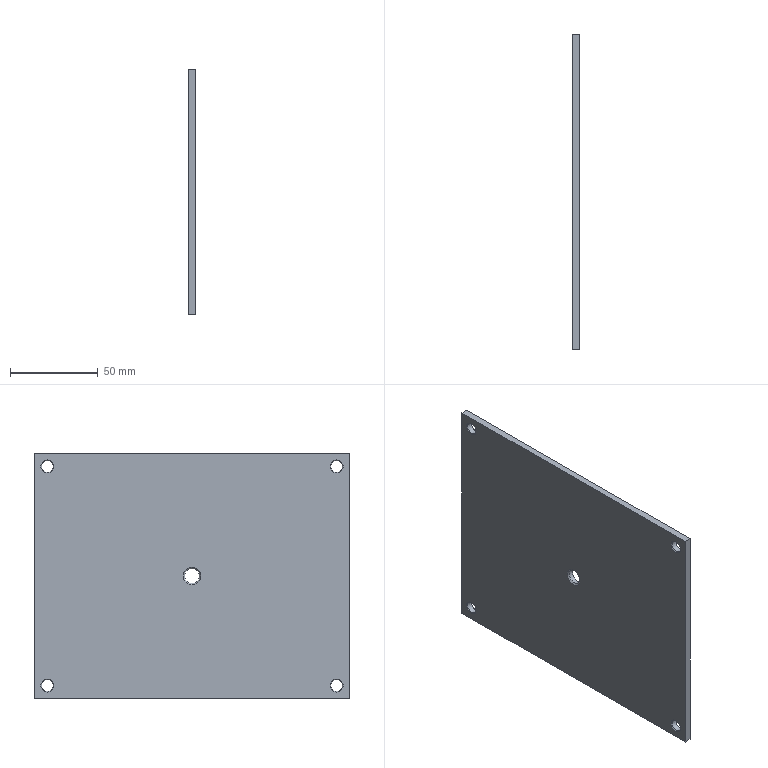Part | NX | 1 solid | 21 faces | box 4 x 180 x 140 mm | volume 99996 mm3 | cone 10 | plane 6 | cylinder 5 | commonest cylinder face diameters 6.6 x4 8.5 x1
STEP:
#1=CARTESIAN_POINT('',(2.,90.,-70.));
#2=VERTEX_POINT('',#1);
#3=CARTESIAN_POINT('',(2.,-90.,-70.));
#4=VERTEX_POINT('',#3);
#5=CARTESIAN_POINT('',(2.,90.,-70.));
#6=DIRECTION('',(0.,-1.,0.));
#7=VECTOR('',#6,1.);
#8=LINE('',#5,#7);
#9=EDGE_CURVE('',#2,#4,#8,.T.);
#10=ORIENTED_EDGE('',*,*,#9,.F.);
#11=CARTESIAN_POINT('',(6.,90.,-70.));
#12=VERTEX_POINT('',#11);
#13=CARTESIAN_POINT('',(6.,90.,-70.));
#14=DIRECTION('',(-1.,0.,0.));
#15=VECTOR('',#14,1.);
#16=LINE('',#13,#15);
#17=EDGE_CURVE('',#12,#2,#16,.T.);
#18=ORIENTED_EDGE('',*,*,#17,.F.);
#19=CARTESIAN_POINT('',(6.,-90.,-70.));
#20=VERTEX_POINT('',#19);
#21=CARTESIAN_POINT('',(6.,90.,-70.));
#22=DIRECTION('',(0.,-1.,0.));
#23=VECTOR('',#22,1.);
#24=LINE('',#21,#23);
#25=EDGE_CURVE('',#12,#20,#24,.T.);
#26=ORIENTED_EDGE('',*,*,#25,.T.);
#27=CARTESIAN_POINT('',(6.,-90.,-70.));
#28=DIRECTION('',(-1.,0.,0.));
#29=VECTOR('',#28,1.);
#30=LINE('',#27,#29);
#31=EDGE_CURVE('',#20,#4,#30,.T.);
#32=ORIENTED_EDGE('',*,*,#31,.T.);
#33=EDGE_LOOP('',(#10,#18,#26,#32));
#34=FACE_OUTER_BOUND('',#33,.T.);
#35=CARTESIAN_POINT('',(6.,90.,-70.));
#36=DIRECTION('',(0.,0.,-1.));
#37=DIRECTION('',(0.,-1.,0.));
#38=AXIS2_PLACEMENT_3D('',#35,#36,#37);
#39=PLANE('',#38);
#40=ADVANCED_FACE('',(#34),#39,.T.);
#41=CARTESIAN_POINT('',(2.,-90.,70.));
#42=VERTEX_POINT('',#41);
#43=CARTESIAN_POINT('',(2.,-90.,-70.));
#44=DIRECTION('',(0.,0.,1.));
#45=VECTOR('',#44,1.);
#46=LINE('',#43,#45);
#47=EDGE_CURVE('',#4,#42,#46,.T.);
#48=ORIENTED_EDGE('',*,*,#47,.F.);
#49=ORIENTED_EDGE('',*,*,#31,.F.);
#50=CARTESIAN_POINT('',(6.,-90.,70.));
#51=VERTEX_POINT('',#50);
#52=CARTESIAN_POINT('',(6.,-90.,-70.));
#53=DIRECTION('',(0.,0.,1.));
#54=VECTOR('',#53,1.);
#55=LINE('',#52,#54);
#56=EDGE_CURVE('',#20,#51,#55,.T.);
#57=ORIENTED_EDGE('',*,*,#56,.T.);
#58=CARTESIAN_POINT('',(6.,-90.,70.));
#59=DIRECTION('',(-1.,0.,0.));
#60=VECTOR('',#59,1.);
#61=LINE('',#58,#60);
#62=EDGE_CURVE('',#51,#42,#61,.T.);
#63=ORIENTED_EDGE('',*,*,#62,.T.);
#64=EDGE_LOOP('',(#48,#49,#57,#63));
#65=FACE_OUTER_BOUND('',#64,.T.);
#66=CARTESIAN_POINT('',(6.,-90.,-70.));
#67=DIRECTION('',(0.,-1.,0.));
#68=DIRECTION('',(0.,0.,1.));
#69=AXIS2_PLACEMENT_3D('',#66,#67,#68);
#70=PLANE('',#69);
#71=ADVANCED_FACE('',(#65),#70,.T.);
#72=CARTESIAN_POINT('',(2.,90.,70.));
#73=VERTEX_POINT('',#72);
#74=CARTESIAN_POINT('',(2.,-90.,70.));
#75=DIRECTION('',(0.,1.,0.));
#76=VECTOR('',#75,1.);
#77=LINE('',#74,#76);
#78=EDGE_CURVE('',#42,#73,#77,.T.);
#79=ORIENTED_EDGE('',*,*,#78,.F.);
#80=ORIENTED_EDGE('',*,*,#62,.F.);
#81=CARTESIAN_POINT('',(6.,90.,70.));
#82=VERTEX_POINT('',#81);
#83=CARTESIAN_POINT('',(6.,-90.,70.));
#84=DIRECTION('',(0.,1.,0.));
#85=VECTOR('',#84,1.);
#86=LINE('',#83,#85);
#87=EDGE_CURVE('',#51,#82,#86,.T.);
#88=ORIENTED_EDGE('',*,*,#87,.T.);
#89=CARTESIAN_POINT('',(6.,90.,70.));
#90=DIRECTION('',(-1.,0.,0.));
#91=VECTOR('',#90,1.);
#92=LINE('',#89,#91);
#93=EDGE_CURVE('',#82,#73,#92,.T.);
#94=ORIENTED_EDGE('',*,*,#93,.T.);
#95=EDGE_LOOP('',(#79,#80,#88,#94));
#96=FACE_OUTER_BOUND('',#95,.T.);
#97=CARTESIAN_POINT('',(6.,-90.,70.));
#98=DIRECTION('',(0.,0.,1.));
#99=DIRECTION('',(0.,1.,0.));
#100=AXIS2_PLACEMENT_3D('',#97,#98,#99);
#101=PLANE('',#100);
#102=ADVANCED_FACE('',(#96),#101,.T.);
#103=CARTESIAN_POINT('',(2.,90.,70.));
#104=DIRECTION('',(0.,0.,-1.));
#105=VECTOR('',#104,1.);
#106=LINE('',#103,#105);
#107=EDGE_CURVE('',#73,#2,#106,.T.);
#108=ORIENTED_EDGE('',*,*,#107,.F.);
#109=ORIENTED_EDGE('',*,*,#93,.F.);
#110=CARTESIAN_POINT('',(6.,90.,70.));
#111=DIRECTION('',(0.,0.,-1.));
#112=VECTOR('',#111,1.);
#113=LINE('',#110,#112);
#114=EDGE_CURVE('',#82,#12,#113,.T.);
#115=ORIENTED_EDGE('',*,*,#114,.T.);
#116=ORIENTED_EDGE('',*,*,#17,.T.);
#117=EDGE_LOOP('',(#108,#109,#115,#116));
#118=FACE_OUTER_BOUND('',#117,.T.);
#119=CARTESIAN_POINT('',(6.,90.,70.));
#120=DIRECTION('',(0.,1.,0.));
#121=DIRECTION('',(0.,0.,-1.));
#122=AXIS2_PLACEMENT_3D('',#119,#120,#121);
#123=PLANE('',#122);
#124=ADVANCED_FACE('',(#118),#123,.T.);
#125=CARTESIAN_POINT('',(6.,0.,5.));
#126=VERTEX_POINT('',#125);
#127=CARTESIAN_POINT('',(6.,0.,0.));
#128=DIRECTION('',(-1.,0.,0.));
#129=DIRECTION('',(0.,0.,1.));
#130=AXIS2_PLACEMENT_3D('',#127,#128,#129);
#131=CIRCLE('',#130,5.);
#132=EDGE_CURVE('',#126,#126,#131,.T.);
#133=ORIENTED_EDGE('',*,*,#132,.T.);
#134=EDGE_LOOP('',(#133));
#135=FACE_BOUND('',#134,.T.);
#136=CARTESIAN_POINT('',(6.,82.5,66.2));
#137=VERTEX_POINT('',#136);
#138=CARTESIAN_POINT('',(6.,82.5,62.5));
#139=DIRECTION('',(-1.,0.,0.));
#140=DIRECTION('',(0.,0.,1.));
#141=AXIS2_PLACEMENT_3D('',#138,#139,#140);
#142=CIRCLE('',#141,3.7);
#143=EDGE_CURVE('',#137,#137,#142,.T.);
#144=ORIENTED_EDGE('',*,*,#143,.T.);
#145=EDGE_LOOP('',(#144));
#146=FACE_BOUND('',#145,.T.);
#147=CARTESIAN_POINT('',(6.,82.5,-58.8));
#148=VERTEX_POINT('',#147);
#149=CARTESIAN_POINT('',(6.,82.5,-62.5));
#150=DIRECTION('',(-1.,0.,0.));
#151=DIRECTION('',(0.,0.,1.));
#152=AXIS2_PLACEMENT_3D('',#149,#150,#151);
#153=CIRCLE('',#152,3.7);
#154=EDGE_CURVE('',#148,#148,#153,.T.);
#155=ORIENTED_EDGE('',*,*,#154,.T.);
#156=EDGE_LOOP('',(#155));
#157=FACE_BOUND('',#156,.T.);
#158=CARTESIAN_POINT('',(6.,-82.5,66.2));
#159=VERTEX_POINT('',#158);
#160=CARTESIAN_POINT('',(6.,-82.5,62.5));
#161=DIRECTION('',(-1.,0.,0.));
#162=DIRECTION('',(0.,0.,1.));
#163=AXIS2_PLACEMENT_3D('',#160,#161,#162);
#164=CIRCLE('',#163,3.7);
#165=EDGE_CURVE('',#159,#159,#164,.T.);
#166=ORIENTED_EDGE('',*,*,#165,.T.);
#167=EDGE_LOOP('',(#166));
#168=FACE_BOUND('',#167,.T.);
#169=CARTESIAN_POINT('',(6.,-82.5,-58.8));
#170=VERTEX_POINT('',#169);
#171=CARTESIAN_POINT('',(6.,-82.5,-62.5));
#172=DIRECTION('',(-1.,0.,0.));
#173=DIRECTION('',(0.,0.,1.));
#174=AXIS2_PLACEMENT_3D('',#171,#172,#173);
#175=CIRCLE('',#174,3.7);
#176=EDGE_CURVE('',#170,#170,#175,.T.);
#177=ORIENTED_EDGE('',*,*,#176,.T.);
#178=EDGE_LOOP('',(#177));
#179=FACE_BOUND('',#178,.T.);
#180=ORIENTED_EDGE('',*,*,#25,.F.);
#181=ORIENTED_EDGE('',*,*,#114,.F.);
#182=ORIENTED_EDGE('',*,*,#87,.F.);
#183=ORIENTED_EDGE('',*,*,#56,.F.);
#184=EDGE_LOOP('',(#180,#181,#182,#183));
#185=FACE_BOUND('',#184,.T.);
#186=CARTESIAN_POINT('',(6.,0.,0.));
#187=DIRECTION('',(-1.,0.,0.));
#188=DIRECTION('',(0.,0.,-1.));
#189=AXIS2_PLACEMENT_3D('',#186,#187,#188);
#190=PLANE('',#189);
#191=ADVANCED_FACE('',(#135,#146,#157,#168,#179,#185),#190,.F.);
#192=CARTESIAN_POINT('',(2.,0.,5.));
#193=VERTEX_POINT('',#192);
#194=CARTESIAN_POINT('',(2.,0.,0.));
#195=DIRECTION('',(1.,0.,0.));
#196=DIRECTION('',(0.,0.,1.));
#197=AXIS2_PLACEMENT_3D('',#194,#195,#196);
#198=CIRCLE('',#197,5.);
#199=EDGE_CURVE('',#193,#193,#198,.T.);
#200=ORIENTED_EDGE('',*,*,#199,.T.);
#201=EDGE_LOOP('',(#200));
#202=FACE_BOUND('',#201,.T.);
#203=CARTESIAN_POINT('',(2.,82.5,66.2));
#204=VERTEX_POINT('',#203);
#205=CARTESIAN_POINT('',(2.,82.5,62.5));
#206=DIRECTION('',(1.,0.,0.));
#207=DIRECTION('',(0.,0.,1.));
#208=AXIS2_PLACEMENT_3D('',#205,#206,#207);
#209=CIRCLE('',#208,3.7);
#210=EDGE_CURVE('',#204,#204,#209,.T.);
#211=ORIENTED_EDGE('',*,*,#210,.T.);
#212=EDGE_LOOP('',(#211));
#213=FACE_BOUND('',#212,.T.);
#214=CARTESIAN_POINT('',(2.,82.5,-58.8));
#215=VERTEX_POINT('',#214);
#216=CARTESIAN_POINT('',(2.,82.5,-62.5));
#217=DIRECTION('',(1.,0.,0.));
#218=DIRECTION('',(0.,0.,1.));
#219=AXIS2_PLACEMENT_3D('',#216,#217,#218);
#220=CIRCLE('',#219,3.7);
#221=EDGE_CURVE('',#215,#215,#220,.T.);
#222=ORIENTED_EDGE('',*,*,#221,.T.);
#223=EDGE_LOOP('',(#222));
#224=FACE_BOUND('',#223,.T.);
#225=CARTESIAN_POINT('',(2.,-82.5,66.2));
#226=VERTEX_POINT('',#225);
#227=CARTESIAN_POINT('',(2.,-82.5,62.5));
#228=DIRECTION('',(1.,0.,0.));
#229=DIRECTION('',(0.,0.,1.));
#230=AXIS2_PLACEMENT_3D('',#227,#228,#229);
#231=CIRCLE('',#230,3.7);
#232=EDGE_CURVE('',#226,#226,#231,.T.);
#233=ORIENTED_EDGE('',*,*,#232,.T.);
#234=EDGE_LOOP('',(#233));
#235=FACE_BOUND('',#234,.T.);
#236=CARTESIAN_POINT('',(2.,-82.5,-58.8));
#237=VERTEX_POINT('',#236);
#238=CARTESIAN_POINT('',(2.,-82.5,-62.5));
#239=DIRECTION('',(1.,0.,0.));
#240=DIRECTION('',(0.,0.,1.));
#241=AXIS2_PLACEMENT_3D('',#238,#239,#240);
#242=CIRCLE('',#241,3.7);
#243=EDGE_CURVE('',#237,#237,#242,.T.);
#244=ORIENTED_EDGE('',*,*,#243,.T.);
#245=EDGE_LOOP('',(#244));
#246=FACE_BOUND('',#245,.T.);
#247=ORIENTED_EDGE('',*,*,#9,.T.);
#248=ORIENTED_EDGE('',*,*,#47,.T.);
#249=ORIENTED_EDGE('',*,*,#78,.T.);
#250=ORIENTED_EDGE('',*,*,#107,.T.);
#251=EDGE_LOOP('',(#247,#248,#249,#250));
#252=FACE_BOUND('',#251,.T.);
#253=CARTESIAN_POINT('',(2.,0.,0.));
#254=DIRECTION('',(-1.,0.,0.));
#255=DIRECTION('',(0.,0.,-1.));
#256=AXIS2_PLACEMENT_3D('',#253,#254,#255);
#257=PLANE('',#256);
#258=ADVANCED_FACE('',(#202,#213,#224,#235,#246,#252),#257,.T.);
#259=CARTESIAN_POINT('',(5.6,-82.5,-59.2));
#260=VERTEX_POINT('',#259);
#261=CARTESIAN_POINT('',(5.6,-82.5,-62.5));
#262=DIRECTION('',(1.,0.,0.));
#263=DIRECTION('',(0.,0.,1.));
#264=AXIS2_PLACEMENT_3D('',#261,#262,#263);
#265=CIRCLE('',#264,3.3);
#266=EDGE_CURVE('',#260,#260,#265,.T.);
#267=ORIENTED_EDGE('',*,*,#266,.T.);
#268=EDGE_LOOP('',(#267));
#269=FACE_BOUND('',#268,.T.);
#270=CARTESIAN_POINT('',(2.4,-82.5,-59.2));
#271=VERTEX_POINT('',#270);
#272=CARTESIAN_POINT('',(2.4,-82.5,-62.5));
#273=DIRECTION('',(-1.,0.,0.));
#274=DIRECTION('',(0.,0.,1.));
#275=AXIS2_PLACEMENT_3D('',#272,#273,#274);
#276=CIRCLE('',#275,3.3);
#277=EDGE_CURVE('',#271,#271,#276,.T.);
#278=ORIENTED_EDGE('',*,*,#277,.T.);
#279=EDGE_LOOP('',(#278));
#280=FACE_BOUND('',#279,.T.);
#281=CARTESIAN_POINT('',(0.,-82.5,-62.5));
#282=DIRECTION('',(1.,0.,0.));
#283=DIRECTION('',(0.,0.,1.));
#284=AXIS2_PLACEMENT_3D('',#281,#282,#283);
#285=CYLINDRICAL_SURFACE('',#284,3.3);
#286=ADVANCED_FACE('',(#269,#280),#285,.F.);
#287=ORIENTED_EDGE('',*,*,#243,.F.);
#288=EDGE_LOOP('',(#287));
#289=FACE_BOUND('',#288,.T.);
#290=ORIENTED_EDGE('',*,*,#277,.F.);
#291=EDGE_LOOP('',(#290));
#292=FACE_BOUND('',#291,.T.);
#293=CARTESIAN_POINT('',(2.4,-82.5,-62.5));
#294=DIRECTION('',(-1.,0.,0.));
#295=DIRECTION('',(0.,0.,-1.));
#296=AXIS2_PLACEMENT_3D('',#293,#294,#295);
#297=CONICAL_SURFACE('',#296,3.3,45.);
#298=ADVANCED_FACE('',(#289,#292),#297,.F.);
#299=ORIENTED_EDGE('',*,*,#266,.F.);
#300=EDGE_LOOP('',(#299));
#301=FACE_BOUND('',#300,.T.);
#302=ORIENTED_EDGE('',*,*,#176,.F.);
#303=EDGE_LOOP('',(#302));
#304=FACE_BOUND('',#303,.T.);
#305=CARTESIAN_POINT('',(6.,-82.5,-62.5));
#306=DIRECTION('',(1.,0.,0.));
#307=DIRECTION('',(0.,0.,1.));
#308=AXIS2_PLACEMENT_3D('',#305,#306,#307);
#309=CONICAL_SURFACE('',#308,3.7,45.);
#310=ADVANCED_FACE('',(#301,#304),#309,.F.);
#311=CARTESIAN_POINT('',(5.6,-82.5,65.8));
#312=VERTEX_POINT('',#311);
#313=CARTESIAN_POINT('',(5.6,-82.5,62.5));
#314=DIRECTION('',(1.,0.,0.));
#315=DIRECTION('',(0.,0.,1.));
#316=AXIS2_PLACEMENT_3D('',#313,#314,#315);
#317=CIRCLE('',#316,3.3);
#318=EDGE_CURVE('',#312,#312,#317,.T.);
#319=ORIENTED_EDGE('',*,*,#318,.T.);
#320=EDGE_LOOP('',(#319));
#321=FACE_BOUND('',#320,.T.);
#322=CARTESIAN_POINT('',(2.4,-82.5,65.8));
#323=VERTEX_POINT('',#322);
#324=CARTESIAN_POINT('',(2.4,-82.5,62.5));
#325=DIRECTION('',(-1.,0.,0.));
#326=DIRECTION('',(0.,0.,1.));
#327=AXIS2_PLACEMENT_3D('',#324,#325,#326);
#328=CIRCLE('',#327,3.3);
#329=EDGE_CURVE('',#323,#323,#328,.T.);
#330=ORIENTED_EDGE('',*,*,#329,.T.);
#331=EDGE_LOOP('',(#330));
#332=FACE_BOUND('',#331,.T.);
#333=CARTESIAN_POINT('',(0.,-82.5,62.5));
#334=DIRECTION('',(1.,0.,0.));
#335=DIRECTION('',(0.,0.,1.));
#336=AXIS2_PLACEMENT_3D('',#333,#334,#335);
#337=CYLINDRICAL_SURFACE('',#336,3.3);
#338=ADVANCED_FACE('',(#321,#332),#337,.F.);
#339=ORIENTED_EDGE('',*,*,#232,.F.);
#340=EDGE_LOOP('',(#339));
#341=FACE_BOUND('',#340,.T.);
#342=ORIENTED_EDGE('',*,*,#329,.F.);
#343=EDGE_LOOP('',(#342));
#344=FACE_BOUND('',#343,.T.);
#345=CARTESIAN_POINT('',(2.4,-82.5,62.5));
#346=DIRECTION('',(-1.,0.,0.));
#347=DIRECTION('',(0.,0.,-1.));
#348=AXIS2_PLACEMENT_3D('',#345,#346,#347);
#349=CONICAL_SURFACE('',#348,3.3,45.);
#350=ADVANCED_FACE('',(#341,#344),#349,.F.);
#351=ORIENTED_EDGE('',*,*,#318,.F.);
#352=EDGE_LOOP('',(#351));
#353=FACE_BOUND('',#352,.T.);
#354=ORIENTED_EDGE('',*,*,#165,.F.);
#355=EDGE_LOOP('',(#354));
#356=FACE_BOUND('',#355,.T.);
#357=CARTESIAN_POINT('',(6.,-82.5,62.5));
#358=DIRECTION('',(1.,0.,0.));
#359=DIRECTION('',(0.,0.,1.));
#360=AXIS2_PLACEMENT_3D('',#357,#358,#359);
#361=CONICAL_SURFACE('',#360,3.7,45.);
#362=ADVANCED_FACE('',(#353,#356),#361,.F.);
#363=CARTESIAN_POINT('',(5.6,82.5,-59.2));
#364=VERTEX_POINT('',#363);
#365=CARTESIAN_POINT('',(5.6,82.5,-62.5));
#366=DIRECTION('',(1.,0.,0.));
#367=DIRECTION('',(0.,0.,1.));
#368=AXIS2_PLACEMENT_3D('',#365,#366,#367);
#369=CIRCLE('',#368,3.3);
#370=EDGE_CURVE('',#364,#364,#369,.T.);
#371=ORIENTED_EDGE('',*,*,#370,.T.);
#372=EDGE_LOOP('',(#371));
#373=FACE_BOUND('',#372,.T.);
#374=CARTESIAN_POINT('',(2.4,82.5,-59.2));
#375=VERTEX_POINT('',#374);
#376=CARTESIAN_POINT('',(2.4,82.5,-62.5));
#377=DIRECTION('',(-1.,0.,0.));
#378=DIRECTION('',(0.,0.,1.));
#379=AXIS2_PLACEMENT_3D('',#376,#377,#378);
#380=CIRCLE('',#379,3.3);
#381=EDGE_CURVE('',#375,#375,#380,.T.);
#382=ORIENTED_EDGE('',*,*,#381,.T.);
#383=EDGE_LOOP('',(#382));
#384=FACE_BOUND('',#383,.T.);
#385=CARTESIAN_POINT('',(0.,82.5,-62.5));
#386=DIRECTION('',(1.,0.,0.));
#387=DIRECTION('',(0.,0.,1.));
#388=AXIS2_PLACEMENT_3D('',#385,#386,#387);
#389=CYLINDRICAL_SURFACE('',#388,3.3);
#390=ADVANCED_FACE('',(#373,#384),#389,.F.);
#391=ORIENTED_EDGE('',*,*,#221,.F.);
#392=EDGE_LOOP('',(#391));
#393=FACE_BOUND('',#392,.T.);
#394=ORIENTED_EDGE('',*,*,#381,.F.);
#395=EDGE_LOOP('',(#394));
#396=FACE_BOUND('',#395,.T.);
#397=CARTESIAN_POINT('',(2.4,82.5,-62.5));
#398=DIRECTION('',(-1.,0.,0.));
#399=DIRECTION('',(0.,0.,-1.));
#400=AXIS2_PLACEMENT_3D('',#397,#398,#399);
#401=CONICAL_SURFACE('',#400,3.3,45.);
#402=ADVANCED_FACE('',(#393,#396),#401,.F.);
#403=ORIENTED_EDGE('',*,*,#370,.F.);
#404=EDGE_LOOP('',(#403));
#405=FACE_BOUND('',#404,.T.);
#406=ORIENTED_EDGE('',*,*,#154,.F.);
#407=EDGE_LOOP('',(#406));
#408=FACE_BOUND('',#407,.T.);
#409=CARTESIAN_POINT('',(6.,82.5,-62.5));
#410=DIRECTION('',(1.,0.,0.));
#411=DIRECTION('',(0.,0.,1.));
#412=AXIS2_PLACEMENT_3D('',#409,#410,#411);
#413=CONICAL_SURFACE('',#412,3.7,45.);
#414=ADVANCED_FACE('',(#405,#408),#413,.F.);
#415=CARTESIAN_POINT('',(5.6,82.5,65.8));
#416=VERTEX_POINT('',#415);
#417=CARTESIAN_POINT('',(5.6,82.5,62.5));
#418=DIRECTION('',(1.,0.,0.));
#419=DIRECTION('',(0.,0.,1.));
#420=AXIS2_PLACEMENT_3D('',#417,#418,#419);
#421=CIRCLE('',#420,3.3);
#422=EDGE_CURVE('',#416,#416,#421,.T.);
#423=ORIENTED_EDGE('',*,*,#422,.T.);
#424=EDGE_LOOP('',(#423));
#425=FACE_BOUND('',#424,.T.);
#426=CARTESIAN_POINT('',(2.4,82.5,65.8));
#427=VERTEX_POINT('',#426);
#428=CARTESIAN_POINT('',(2.4,82.5,62.5));
#429=DIRECTION('',(-1.,0.,0.));
#430=DIRECTION('',(0.,0.,1.));
#431=AXIS2_PLACEMENT_3D('',#428,#429,#430);
#432=CIRCLE('',#431,3.3);
#433=EDGE_CURVE('',#427,#427,#432,.T.);
#434=ORIENTED_EDGE('',*,*,#433,.T.);
#435=EDGE_LOOP('',(#434));
#436=FACE_BOUND('',#435,.T.);
#437=CARTESIAN_POINT('',(0.,82.5,62.5));
#438=DIRECTION('',(1.,0.,0.));
#439=DIRECTION('',(0.,0.,1.));
#440=AXIS2_PLACEMENT_3D('',#437,#438,#439);
#441=CYLINDRICAL_SURFACE('',#440,3.3);
#442=ADVANCED_FACE('',(#425,#436),#441,.F.);
#443=ORIENTED_EDGE('',*,*,#210,.F.);
#444=EDGE_LOOP('',(#443));
#445=FACE_BOUND('',#444,.T.);
#446=ORIENTED_EDGE('',*,*,#433,.F.);
#447=EDGE_LOOP('',(#446));
#448=FACE_BOUND('',#447,.T.);
#449=CARTESIAN_POINT('',(2.4,82.5,62.5));
#450=DIRECTION('',(-1.,0.,0.));
#451=DIRECTION('',(0.,0.,-1.));
#452=AXIS2_PLACEMENT_3D('',#449,#450,#451);
#453=CONICAL_SURFACE('',#452,3.3,45.);
#454=ADVANCED_FACE('',(#445,#448),#453,.F.);
#455=ORIENTED_EDGE('',*,*,#422,.F.);
#456=EDGE_LOOP('',(#455));
#457=FACE_BOUND('',#456,.T.);
#458=ORIENTED_EDGE('',*,*,#143,.F.);
#459=EDGE_LOOP('',(#458));
#460=FACE_BOUND('',#459,.T.);
#461=CARTESIAN_POINT('',(6.,82.5,62.5));
#462=DIRECTION('',(1.,0.,0.));
#463=DIRECTION('',(0.,0.,1.));
#464=AXIS2_PLACEMENT_3D('',#461,#462,#463);
#465=CONICAL_SURFACE('',#464,3.7,45.);
#466=ADVANCED_FACE('',(#457,#460),#465,.F.);
#467=CARTESIAN_POINT('',(5.25,0.,4.25));
#468=VERTEX_POINT('',#467);
#469=CARTESIAN_POINT('',(5.25,0.,0.));
#470=DIRECTION('',(1.,0.,0.));
#471=DIRECTION('',(0.,0.,1.));
#472=AXIS2_PLACEMENT_3D('',#469,#470,#471);
#473=CIRCLE('',#472,4.25);
#474=EDGE_CURVE('',#468,#468,#473,.T.);
#475=ORIENTED_EDGE('',*,*,#474,.T.);
#476=EDGE_LOOP('',(#475));
#477=FACE_BOUND('',#476,.T.);
#478=CARTESIAN_POINT('',(2.75,0.,4.25));
#479=VERTEX_POINT('',#478);
#480=CARTESIAN_POINT('',(2.75,0.,0.));
#481=DIRECTION('',(-1.,0.,0.));
#482=DIRECTION('',(0.,0.,1.));
#483=AXIS2_PLACEMENT_3D('',#480,#481,#482);
#484=CIRCLE('',#483,4.25);
#485=EDGE_CURVE('',#479,#479,#484,.T.);
#486=ORIENTED_EDGE('',*,*,#485,.T.);
#487=EDGE_LOOP('',(#486));
#488=FACE_BOUND('',#487,.T.);
#489=CARTESIAN_POINT('',(0.,0.,0.));
#490=DIRECTION('',(1.,0.,0.));
#491=DIRECTION('',(0.,0.,1.));
#492=AXIS2_PLACEMENT_3D('',#489,#490,#491);
#493=CYLINDRICAL_SURFACE('',#492,4.25);
#494=ADVANCED_FACE('',(#477,#488),#493,.F.);
#495=ORIENTED_EDGE('',*,*,#199,.F.);
#496=EDGE_LOOP('',(#495));
#497=FACE_BOUND('',#496,.T.);
#498=ORIENTED_EDGE('',*,*,#485,.F.);
#499=EDGE_LOOP('',(#498));
#500=FACE_BOUND('',#499,.T.);
#501=CARTESIAN_POINT('',(2.75,0.,0.));
#502=DIRECTION('',(-1.,0.,0.));
#503=DIRECTION('',(0.,0.,-1.));
#504=AXIS2_PLACEMENT_3D('',#501,#502,#503);
#505=CONICAL_SURFACE('',#504,4.25,45.);
#506=ADVANCED_FACE('',(#497,#500),#505,.F.);
#507=ORIENTED_EDGE('',*,*,#474,.F.);
#508=EDGE_LOOP('',(#507));
#509=FACE_BOUND('',#508,.T.);
#510=ORIENTED_EDGE('',*,*,#132,.F.);
#511=EDGE_LOOP('',(#510));
#512=FACE_BOUND('',#511,.T.);
#513=CARTESIAN_POINT('',(6.,0.,0.));
#514=DIRECTION('',(1.,0.,0.));
#515=DIRECTION('',(0.,0.,1.));
#516=AXIS2_PLACEMENT_3D('',#513,#514,#515);
#517=CONICAL_SURFACE('',#516,5.,45.);
#518=ADVANCED_FACE('',(#509,#512),#517,.F.);
#519=CLOSED_SHELL('',(#40,#71,#102,#124,#191,#258,#286,#298,#310,#338,#350,#362,#390,#402,#414,#442,#454,#466,#494,#506,#518));
#520=MANIFOLD_SOLID_BREP('',#519);
#521=(LENGTH_UNIT()NAMED_UNIT(*)SI_UNIT(.MILLI.,.METRE.));
#522=UNCERTAINTY_MEASURE_WITH_UNIT(LENGTH_MEASURE(0.00002),#521,'','');
#523=(NAMED_UNIT(*)PLANE_ANGLE_UNIT()SI_UNIT($,.RADIAN.));
#524=PLANE_ANGLE_MEASURE_WITH_UNIT(PLANE_ANGLE_MEASURE(0.01745),#523);
#525=DIMENSIONAL_EXPONENTS(0.,0.,0.,0.,0.,0.,0.);
#526=(CONVERSION_BASED_UNIT('DEGREE',#524)NAMED_UNIT(#525)PLANE_ANGLE_UNIT());
#527=(NAMED_UNIT(*)SI_UNIT($,.STERADIAN.)SOLID_ANGLE_UNIT());
#528=(GEOMETRIC_REPRESENTATION_CONTEXT(3)GLOBAL_UNCERTAINTY_ASSIGNED_CONTEXT((#522))GLOBAL_UNIT_ASSIGNED_CONTEXT((#521,#526,#527))REPRESENTATION_CONTEXT('',''));
#529=ADVANCED_BREP_SHAPE_REPRESENTATION('',(#520),#528);